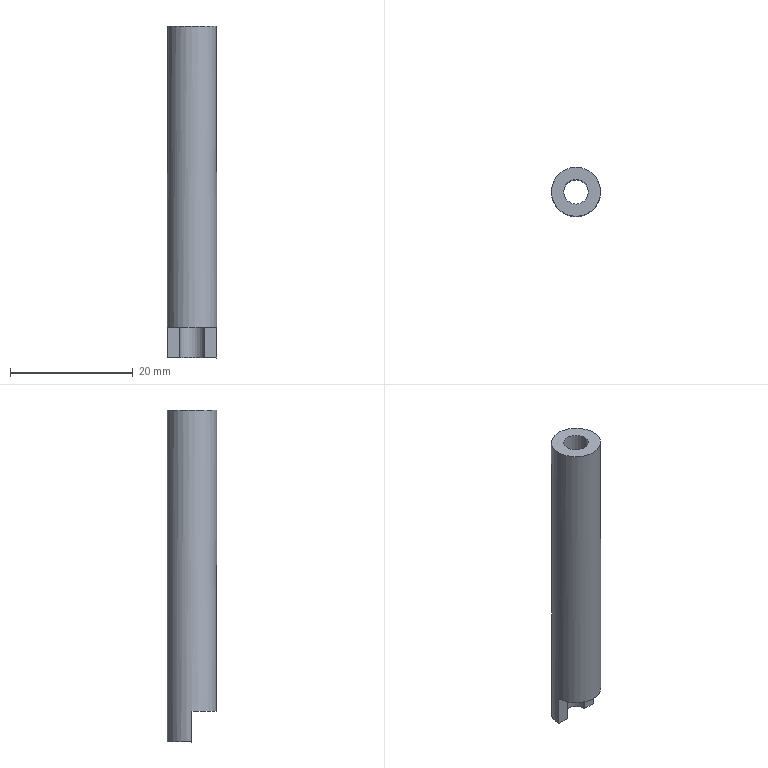Part | NX | features solid 2 | 1 solid | 7 faces | box 8 x 8.001 x 54.001 mm | volume 1941 mm3 | plane 5 | cylinder 2 | commonest cylinder face diameters 4.003 x1 8 x1
STEP:
#1=CARTESIAN_POINT('',(-194.023,-39.723,50.998));
#2=VERTEX_POINT('',#1);
#3=CARTESIAN_POINT('',(-186.023,-39.723,50.998));
#4=VERTEX_POINT('',#3);
#5=CARTESIAN_POINT('',(-190.023,-39.723,50.998));
#6=DIRECTION('',(-0.000001665,0.00001617,-1.));
#7=DIRECTION('',(1.,0.,-0.000001665));
#8=AXIS2_PLACEMENT_3D('',#5,#6,#7);
#9=CIRCLE('',#8,4.);
#10=EDGE_CURVE('',#2,#4,#9,.T.);
#11=ORIENTED_EDGE('',*,*,#10,.T.);
#12=CARTESIAN_POINT('',(-188.022,-39.723,50.998));
#13=VERTEX_POINT('',#12);
#14=CARTESIAN_POINT('',(-185.023,-39.723,50.998));
#15=DIRECTION('',(-1.,0.,0.000001665));
#16=VECTOR('',#15,1000.);
#17=LINE('',#14,#16);
#18=EDGE_CURVE('',#4,#13,#17,.T.);
#19=ORIENTED_EDGE('',*,*,#18,.T.);
#20=CARTESIAN_POINT('',(-192.025,-39.723,50.998));
#21=VERTEX_POINT('',#20);
#22=CARTESIAN_POINT('',(-190.023,-39.723,50.998));
#23=DIRECTION('',(-0.000001665,0.00001617,-1.));
#24=DIRECTION('',(1.,0.,-0.000001665));
#25=AXIS2_PLACEMENT_3D('',#22,#23,#24);
#26=CIRCLE('',#25,2.002);
#27=EDGE_CURVE('',#21,#13,#26,.T.);
#28=ORIENTED_EDGE('',*,*,#27,.F.);
#29=CARTESIAN_POINT('',(-185.023,-39.723,50.998));
#30=DIRECTION('',(-1.,0.,0.000001665));
#31=VECTOR('',#30,1000.);
#32=LINE('',#29,#31);
#33=EDGE_CURVE('',#21,#2,#32,.T.);
#34=ORIENTED_EDGE('',*,*,#33,.T.);
#35=EDGE_LOOP('',(#11,#19,#28,#34));
#36=FACE_BOUND('',#35,.T.);
#37=CARTESIAN_POINT('',(-190.023,-39.723,50.998));
#38=DIRECTION('',(-0.000001665,0.00001617,-1.));
#39=DIRECTION('',(0.,-1.,-0.00001617));
#40=AXIS2_PLACEMENT_3D('',#37,#38,#39);
#41=PLANE('',#40);
#42=ADVANCED_FACE('',(#36),#41,.T.);
#43=ORIENTED_EDGE('',*,*,#10,.F.);
#44=CARTESIAN_POINT('',(-194.023,-39.723,55.998));
#45=VERTEX_POINT('',#44);
#46=CARTESIAN_POINT('',(-194.023,-39.723,50.998));
#47=DIRECTION('',(0.000001665,-0.00001617,1.));
#48=VECTOR('',#47,1000.);
#49=LINE('',#46,#48);
#50=EDGE_CURVE('',#2,#45,#49,.T.);
#51=ORIENTED_EDGE('',*,*,#50,.T.);
#52=CARTESIAN_POINT('',(-186.023,-39.723,55.998));
#53=VERTEX_POINT('',#52);
#54=CARTESIAN_POINT('',(-190.023,-39.723,55.998));
#55=DIRECTION('',(-0.000001665,0.00001617,-1.));
#56=DIRECTION('',(0.,-1.,-0.00001617));
#57=AXIS2_PLACEMENT_3D('',#54,#55,#56);
#58=CIRCLE('',#57,4.);
#59=EDGE_CURVE('',#53,#45,#58,.T.);
#60=ORIENTED_EDGE('',*,*,#59,.F.);
#61=CARTESIAN_POINT('',(-186.023,-39.723,50.998));
#62=DIRECTION('',(0.000001665,-0.00001617,1.));
#63=VECTOR('',#62,1000.);
#64=LINE('',#61,#63);
#65=EDGE_CURVE('',#53,#4,#64,.F.);
#66=ORIENTED_EDGE('',*,*,#65,.T.);
#67=EDGE_LOOP('',(#43,#51,#60,#66));
#68=FACE_BOUND('',#67,.T.);
#69=CARTESIAN_POINT('',(-190.023,-35.724,104.999));
#70=VERTEX_POINT('',#69);
#71=CARTESIAN_POINT('',(-190.023,-39.724,104.999));
#72=DIRECTION('',(0.000001665,-0.00001617,1.));
#73=DIRECTION('',(0.,1.,0.00001617));
#74=AXIS2_PLACEMENT_3D('',#71,#72,#73);
#75=CIRCLE('',#74,4.);
#76=EDGE_CURVE('',#70,#70,#75,.F.);
#77=ORIENTED_EDGE('',*,*,#76,.T.);
#78=EDGE_LOOP('',(#77));
#79=FACE_BOUND('',#78,.T.);
#80=CARTESIAN_POINT('',(-190.023,-39.723,50.998));
#81=DIRECTION('',(0.000001665,-0.00001617,1.));
#82=DIRECTION('',(0.,1.,0.00001617));
#83=AXIS2_PLACEMENT_3D('',#80,#81,#82);
#84=CYLINDRICAL_SURFACE('',#83,4.);
#85=ADVANCED_FACE('',(#68,#79),#84,.T.);
#86=CARTESIAN_POINT('',(-190.023,-37.722,104.999));
#87=VERTEX_POINT('',#86);
#88=CARTESIAN_POINT('',(-190.023,-39.724,104.999));
#89=DIRECTION('',(0.000001665,-0.00001617,1.));
#90=DIRECTION('',(0.,1.,0.00001617));
#91=AXIS2_PLACEMENT_3D('',#88,#89,#90);
#92=CIRCLE('',#91,2.002);
#93=EDGE_CURVE('',#87,#87,#92,.F.);
#94=ORIENTED_EDGE('',*,*,#93,.T.);
#95=EDGE_LOOP('',(#94));
#96=FACE_BOUND('',#95,.T.);
#97=ORIENTED_EDGE('',*,*,#76,.F.);
#98=EDGE_LOOP('',(#97));
#99=FACE_BOUND('',#98,.T.);
#100=CARTESIAN_POINT('',(3849.977,4.198,104.993));
#101=DIRECTION('',(0.000001665,-0.00001617,1.));
#102=DIRECTION('',(-1.,0.,0.000001665));
#103=AXIS2_PLACEMENT_3D('',#100,#101,#102);
#104=PLANE('',#103);
#105=ADVANCED_FACE('',(#96,#99),#104,.T.);
#106=CARTESIAN_POINT('',(-192.025,-39.723,55.998));
#107=VERTEX_POINT('',#106);
#108=CARTESIAN_POINT('',(-192.025,-39.723,50.998));
#109=DIRECTION('',(0.000001665,-0.00001617,1.));
#110=VECTOR('',#109,1000.);
#111=LINE('',#108,#110);
#112=EDGE_CURVE('',#21,#107,#111,.T.);
#113=ORIENTED_EDGE('',*,*,#112,.F.);
#114=ORIENTED_EDGE('',*,*,#27,.T.);
#115=CARTESIAN_POINT('',(-188.022,-39.723,55.998));
#116=VERTEX_POINT('',#115);
#117=CARTESIAN_POINT('',(-188.022,-39.723,50.998));
#118=DIRECTION('',(0.000001665,-0.00001617,1.));
#119=VECTOR('',#118,1000.);
#120=LINE('',#117,#119);
#121=EDGE_CURVE('',#116,#13,#120,.F.);
#122=ORIENTED_EDGE('',*,*,#121,.F.);
#123=CARTESIAN_POINT('',(-190.023,-39.723,55.998));
#124=DIRECTION('',(-0.000001665,0.00001617,-1.));
#125=DIRECTION('',(0.,-1.,-0.00001617));
#126=AXIS2_PLACEMENT_3D('',#123,#124,#125);
#127=CIRCLE('',#126,2.002);
#128=EDGE_CURVE('',#116,#107,#127,.T.);
#129=ORIENTED_EDGE('',*,*,#128,.T.);
#130=EDGE_LOOP('',(#113,#114,#122,#129));
#131=FACE_BOUND('',#130,.T.);
#132=ORIENTED_EDGE('',*,*,#93,.F.);
#133=EDGE_LOOP('',(#132));
#134=FACE_BOUND('',#133,.T.);
#135=CARTESIAN_POINT('',(-190.023,-39.723,50.998));
#136=DIRECTION('',(0.000001665,-0.00001617,1.));
#137=DIRECTION('',(0.,1.,0.00001617));
#138=AXIS2_PLACEMENT_3D('',#135,#136,#137);
#139=CYLINDRICAL_SURFACE('',#138,2.002);
#140=ADVANCED_FACE('',(#131,#134),#139,.F.);
#141=ORIENTED_EDGE('',*,*,#33,.F.);
#142=ORIENTED_EDGE('',*,*,#112,.T.);
#143=CARTESIAN_POINT('',(-185.023,-39.723,55.998));
#144=DIRECTION('',(-1.,0.,0.000001665));
#145=VECTOR('',#144,1000.);
#146=LINE('',#143,#145);
#147=EDGE_CURVE('',#45,#107,#146,.F.);
#148=ORIENTED_EDGE('',*,*,#147,.F.);
#149=ORIENTED_EDGE('',*,*,#50,.F.);
#150=EDGE_LOOP('',(#141,#142,#148,#149));
#151=FACE_BOUND('',#150,.T.);
#152=CARTESIAN_POINT('',(-185.023,-39.723,50.998));
#153=DIRECTION('',(0.,1.,0.00001617));
#154=DIRECTION('',(0.,0.00001617,-1.));
#155=AXIS2_PLACEMENT_3D('',#152,#153,#154);
#156=PLANE('',#155);
#157=ADVANCED_FACE('',(#151),#156,.F.);
#158=CARTESIAN_POINT('',(-185.023,-39.723,55.998));
#159=DIRECTION('',(-1.,0.,0.000001665));
#160=VECTOR('',#159,1000.);
#161=LINE('',#158,#160);
#162=EDGE_CURVE('',#116,#53,#161,.F.);
#163=ORIENTED_EDGE('',*,*,#162,.F.);
#164=ORIENTED_EDGE('',*,*,#121,.T.);
#165=ORIENTED_EDGE('',*,*,#18,.F.);
#166=ORIENTED_EDGE('',*,*,#65,.F.);
#167=EDGE_LOOP('',(#163,#164,#165,#166));
#168=FACE_BOUND('',#167,.T.);
#169=CARTESIAN_POINT('',(-185.023,-39.723,50.998));
#170=DIRECTION('',(0.,1.,0.00001617));
#171=DIRECTION('',(0.,0.00001617,-1.));
#172=AXIS2_PLACEMENT_3D('',#169,#170,#171);
#173=PLANE('',#172);
#174=ADVANCED_FACE('',(#168),#173,.F.);
#175=ORIENTED_EDGE('',*,*,#59,.T.);
#176=ORIENTED_EDGE('',*,*,#147,.T.);
#177=ORIENTED_EDGE('',*,*,#128,.F.);
#178=ORIENTED_EDGE('',*,*,#162,.T.);
#179=EDGE_LOOP('',(#175,#176,#177,#178));
#180=FACE_BOUND('',#179,.T.);
#181=CARTESIAN_POINT('',(-190.023,-39.723,55.998));
#182=DIRECTION('',(-0.000001665,0.00001617,-1.));
#183=DIRECTION('',(0.,-1.,-0.00001617));
#184=AXIS2_PLACEMENT_3D('',#181,#182,#183);
#185=PLANE('',#184);
#186=ADVANCED_FACE('',(#180),#185,.T.);
#187=CLOSED_SHELL('',(#42,#85,#105,#140,#157,#174,#186));
#188=MANIFOLD_SOLID_BREP('',#187);
#189=(LENGTH_UNIT()NAMED_UNIT(*)SI_UNIT(.MILLI.,.METRE.));
#190=UNCERTAINTY_MEASURE_WITH_UNIT(LENGTH_MEASURE(0.00001),#189,'','');
#191=(NAMED_UNIT(*)PLANE_ANGLE_UNIT()SI_UNIT($,.RADIAN.));
#192=(NAMED_UNIT(*)SI_UNIT($,.STERADIAN.)SOLID_ANGLE_UNIT());
#193=(GEOMETRIC_REPRESENTATION_CONTEXT(3)GLOBAL_UNCERTAINTY_ASSIGNED_CONTEXT((#190))GLOBAL_UNIT_ASSIGNED_CONTEXT((#189,#191,#192))REPRESENTATION_CONTEXT('',''));
#194=ADVANCED_BREP_SHAPE_REPRESENTATION('',(#188),#193);